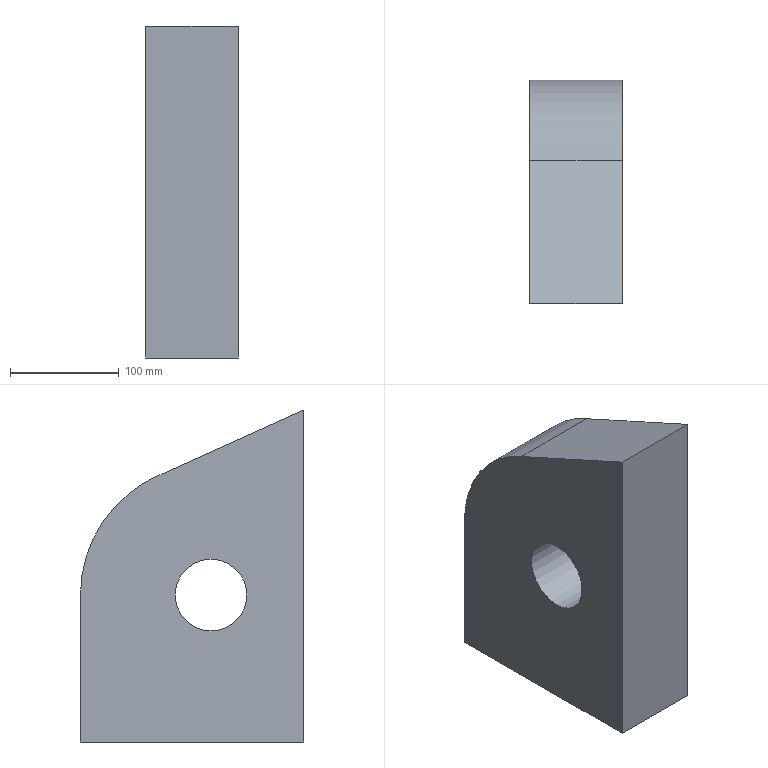Part | NX | features solid 2 | 1 solid | 8 faces | box 85 x 205 x 305 mm | volume 4128992 mm3 | plane 6 | cylinder 2 | commonest cylinder face diameters 66 x1 240 x1
STEP:
#1=CARTESIAN_POINT('',(1245.,1105.,-512.));
#2=VERTEX_POINT('',#1);
#3=CARTESIAN_POINT('',(1245.,1105.,-545.));
#4=DIRECTION('',(1.,0.,0.));
#5=DIRECTION('',(0.,0.,1.));
#6=AXIS2_PLACEMENT_3D('',#3,#4,#5);
#7=CIRCLE('',#6,33.);
#8=EDGE_CURVE('',#2,#2,#7,.F.);
#9=ORIENTED_EDGE('',*,*,#8,.T.);
#10=EDGE_LOOP('',(#9));
#11=FACE_BOUND('',#10,.T.);
#12=CARTESIAN_POINT('',(1330.,1105.,-512.));
#13=VERTEX_POINT('',#12);
#14=CARTESIAN_POINT('',(1330.,1105.,-545.));
#15=DIRECTION('',(1.,0.,0.));
#16=DIRECTION('',(0.,0.,1.));
#17=AXIS2_PLACEMENT_3D('',#14,#15,#16);
#18=CIRCLE('',#17,33.);
#19=EDGE_CURVE('',#13,#13,#18,.F.);
#20=ORIENTED_EDGE('',*,*,#19,.F.);
#21=EDGE_LOOP('',(#20));
#22=FACE_BOUND('',#21,.T.);
#23=CARTESIAN_POINT('',(1495.,1105.,-545.));
#24=DIRECTION('',(-1.,0.,0.));
#25=DIRECTION('',(0.,0.,-1.));
#26=AXIS2_PLACEMENT_3D('',#23,#24,#25);
#27=CYLINDRICAL_SURFACE('',#26,33.);
#28=ADVANCED_FACE('',(#11,#22),#27,.F.);
#29=CARTESIAN_POINT('',(1330.,1150.971,-434.155));
#30=VERTEX_POINT('',#29);
#31=CARTESIAN_POINT('',(1245.,1150.971,-434.155));
#32=VERTEX_POINT('',#31);
#33=CARTESIAN_POINT('',(1175.,1150.971,-434.155));
#34=DIRECTION('',(1.,0.,0.));
#35=VECTOR('',#34,1000.);
#36=LINE('',#33,#35);
#37=EDGE_CURVE('',#30,#32,#36,.F.);
#38=ORIENTED_EDGE('',*,*,#37,.F.);
#39=CARTESIAN_POINT('',(1330.,1225.,-545.));
#40=VERTEX_POINT('',#39);
#41=CARTESIAN_POINT('',(1330.,1105.,-545.));
#42=DIRECTION('',(1.,0.,0.));
#43=DIRECTION('',(0.,0.,1.));
#44=AXIS2_PLACEMENT_3D('',#41,#42,#43);
#45=CIRCLE('',#44,120.);
#46=EDGE_CURVE('',#40,#30,#45,.T.);
#47=ORIENTED_EDGE('',*,*,#46,.F.);
#48=CARTESIAN_POINT('',(1245.,1225.,-545.));
#49=VERTEX_POINT('',#48);
#50=CARTESIAN_POINT('',(1175.,1225.,-545.));
#51=DIRECTION('',(-1.,0.,0.));
#52=VECTOR('',#51,1000.);
#53=LINE('',#50,#52);
#54=EDGE_CURVE('',#49,#40,#53,.F.);
#55=ORIENTED_EDGE('',*,*,#54,.F.);
#56=CARTESIAN_POINT('',(1245.,1105.,-545.));
#57=DIRECTION('',(1.,0.,0.));
#58=DIRECTION('',(0.,0.,1.));
#59=AXIS2_PLACEMENT_3D('',#56,#57,#58);
#60=CIRCLE('',#59,120.);
#61=EDGE_CURVE('',#32,#49,#60,.F.);
#62=ORIENTED_EDGE('',*,*,#61,.F.);
#63=EDGE_LOOP('',(#38,#47,#55,#62));
#64=FACE_BOUND('',#63,.T.);
#65=CARTESIAN_POINT('',(1175.,1105.,-545.));
#66=DIRECTION('',(1.,0.,0.));
#67=DIRECTION('',(0.,0.,-1.));
#68=AXIS2_PLACEMENT_3D('',#65,#66,#67);
#69=CYLINDRICAL_SURFACE('',#68,120.);
#70=ADVANCED_FACE('',(#64),#69,.T.);
#71=CARTESIAN_POINT('',(1330.,1225.,-680.));
#72=VERTEX_POINT('',#71);
#73=CARTESIAN_POINT('',(1245.,1225.,-680.));
#74=VERTEX_POINT('',#73);
#75=CARTESIAN_POINT('',(1175.,1225.,-680.));
#76=DIRECTION('',(-1.,0.,0.));
#77=VECTOR('',#76,1000.);
#78=LINE('',#75,#77);
#79=EDGE_CURVE('',#72,#74,#78,.T.);
#80=ORIENTED_EDGE('',*,*,#79,.T.);
#81=CARTESIAN_POINT('',(1245.,1225.,-560.));
#82=DIRECTION('',(0.,0.,1.));
#83=VECTOR('',#82,1000.);
#84=LINE('',#81,#83);
#85=EDGE_CURVE('',#74,#49,#84,.T.);
#86=ORIENTED_EDGE('',*,*,#85,.T.);
#87=ORIENTED_EDGE('',*,*,#54,.T.);
#88=CARTESIAN_POINT('',(1330.,1225.,-560.));
#89=DIRECTION('',(0.,0.,1.));
#90=VECTOR('',#89,1000.);
#91=LINE('',#88,#90);
#92=EDGE_CURVE('',#72,#40,#91,.T.);
#93=ORIENTED_EDGE('',*,*,#92,.F.);
#94=EDGE_LOOP('',(#80,#86,#87,#93));
#95=FACE_BOUND('',#94,.T.);
#96=CARTESIAN_POINT('',(1175.,1225.,-560.));
#97=DIRECTION('',(0.,1.,0.));
#98=DIRECTION('',(-1.,0.,0.));
#99=AXIS2_PLACEMENT_3D('',#96,#97,#98);
#100=PLANE('',#99);
#101=ADVANCED_FACE('',(#95),#100,.T.);
#102=ORIENTED_EDGE('',*,*,#46,.T.);
#103=CARTESIAN_POINT('',(1330.,1020.,-375.));
#104=VERTEX_POINT('',#103);
#105=CARTESIAN_POINT('',(1330.,1177.538,-446.154));
#106=DIRECTION('',(0.,0.9114,-0.4116));
#107=VECTOR('',#106,1000.);
#108=LINE('',#105,#107);
#109=EDGE_CURVE('',#104,#30,#108,.T.);
#110=ORIENTED_EDGE('',*,*,#109,.F.);
#111=CARTESIAN_POINT('',(1330.,1020.,-680.));
#112=VERTEX_POINT('',#111);
#113=CARTESIAN_POINT('',(1330.,1020.,-360.));
#114=DIRECTION('',(0.,0.,-1.));
#115=VECTOR('',#114,1000.);
#116=LINE('',#113,#115);
#117=EDGE_CURVE('',#104,#112,#116,.T.);
#118=ORIENTED_EDGE('',*,*,#117,.T.);
#119=CARTESIAN_POINT('',(1330.,1050.,-680.));
#120=DIRECTION('',(0.,-1.,0.));
#121=VECTOR('',#120,1000.);
#122=LINE('',#119,#121);
#123=EDGE_CURVE('',#72,#112,#122,.T.);
#124=ORIENTED_EDGE('',*,*,#123,.F.);
#125=ORIENTED_EDGE('',*,*,#92,.T.);
#126=EDGE_LOOP('',(#102,#110,#118,#124,#125));
#127=FACE_BOUND('',#126,.T.);
#128=ORIENTED_EDGE('',*,*,#19,.T.);
#129=EDGE_LOOP('',(#128));
#130=FACE_BOUND('',#129,.T.);
#131=CARTESIAN_POINT('',(1330.,1050.,-510.));
#132=DIRECTION('',(-1.,0.,0.));
#133=DIRECTION('',(0.,-1.,0.));
#134=AXIS2_PLACEMENT_3D('',#131,#132,#133);
#135=PLANE('',#134);
#136=ADVANCED_FACE('',(#127,#130),#135,.F.);
#137=CARTESIAN_POINT('',(1245.,1020.,-375.));
#138=VERTEX_POINT('',#137);
#139=CARTESIAN_POINT('',(1245.,1038.757,-383.472));
#140=DIRECTION('',(0.,0.9114,-0.4116));
#141=VECTOR('',#140,1000.);
#142=LINE('',#139,#141);
#143=EDGE_CURVE('',#138,#32,#142,.T.);
#144=ORIENTED_EDGE('',*,*,#143,.T.);
#145=ORIENTED_EDGE('',*,*,#61,.T.);
#146=ORIENTED_EDGE('',*,*,#85,.F.);
#147=CARTESIAN_POINT('',(1245.,1020.,-680.));
#148=VERTEX_POINT('',#147);
#149=CARTESIAN_POINT('',(1245.,1020.,-680.));
#150=DIRECTION('',(0.,-1.,0.));
#151=VECTOR('',#150,1000.);
#152=LINE('',#149,#151);
#153=EDGE_CURVE('',#74,#148,#152,.T.);
#154=ORIENTED_EDGE('',*,*,#153,.T.);
#155=CARTESIAN_POINT('',(1245.,1020.,-501.379));
#156=DIRECTION('',(0.,0.,-1.));
#157=VECTOR('',#156,1000.);
#158=LINE('',#155,#157);
#159=EDGE_CURVE('',#148,#138,#158,.F.);
#160=ORIENTED_EDGE('',*,*,#159,.T.);
#161=EDGE_LOOP('',(#144,#145,#146,#154,#160));
#162=FACE_BOUND('',#161,.T.);
#163=ORIENTED_EDGE('',*,*,#8,.F.);
#164=EDGE_LOOP('',(#163));
#165=FACE_BOUND('',#164,.T.);
#166=CARTESIAN_POINT('',(1245.,1020.,-250.));
#167=DIRECTION('',(-1.,0.,0.));
#168=DIRECTION('',(0.,0.,-1.));
#169=AXIS2_PLACEMENT_3D('',#166,#167,#168);
#170=PLANE('',#169);
#171=ADVANCED_FACE('',(#162,#165),#170,.T.);
#172=CARTESIAN_POINT('',(1380.,1020.,-375.));
#173=DIRECTION('',(1.,0.,0.));
#174=VECTOR('',#173,1000.);
#175=LINE('',#172,#174);
#176=EDGE_CURVE('',#138,#104,#175,.T.);
#177=ORIENTED_EDGE('',*,*,#176,.F.);
#178=ORIENTED_EDGE('',*,*,#159,.F.);
#179=CARTESIAN_POINT('',(1550.,1020.,-680.));
#180=DIRECTION('',(1.,0.,0.));
#181=VECTOR('',#180,1000.);
#182=LINE('',#179,#181);
#183=EDGE_CURVE('',#148,#112,#182,.T.);
#184=ORIENTED_EDGE('',*,*,#183,.T.);
#185=ORIENTED_EDGE('',*,*,#117,.F.);
#186=EDGE_LOOP('',(#177,#178,#184,#185));
#187=FACE_BOUND('',#186,.T.);
#188=CARTESIAN_POINT('',(1550.,1020.,-425.));
#189=DIRECTION('',(0.,-1.,0.));
#190=DIRECTION('',(0.,0.,1.));
#191=AXIS2_PLACEMENT_3D('',#188,#189,#190);
#192=PLANE('',#191);
#193=ADVANCED_FACE('',(#187),#192,.T.);
#194=ORIENTED_EDGE('',*,*,#79,.F.);
#195=ORIENTED_EDGE('',*,*,#123,.T.);
#196=ORIENTED_EDGE('',*,*,#183,.F.);
#197=ORIENTED_EDGE('',*,*,#153,.F.);
#198=EDGE_LOOP('',(#194,#195,#196,#197));
#199=FACE_BOUND('',#198,.T.);
#200=CARTESIAN_POINT('',(80.,-155.,-680.));
#201=DIRECTION('',(0.,0.,1.));
#202=DIRECTION('',(-1.,0.,0.));
#203=AXIS2_PLACEMENT_3D('',#200,#201,#202);
#204=PLANE('',#203);
#205=ADVANCED_FACE('',(#199),#204,.F.);
#206=ORIENTED_EDGE('',*,*,#109,.T.);
#207=ORIENTED_EDGE('',*,*,#37,.T.);
#208=ORIENTED_EDGE('',*,*,#143,.F.);
#209=ORIENTED_EDGE('',*,*,#176,.T.);
#210=EDGE_LOOP('',(#206,#207,#208,#209));
#211=FACE_BOUND('',#210,.T.);
#212=CARTESIAN_POINT('',(1330.,1020.,-375.));
#213=DIRECTION('',(0.,0.4116,0.9114));
#214=DIRECTION('',(0.,0.9114,-0.4116));
#215=AXIS2_PLACEMENT_3D('',#212,#213,#214);
#216=PLANE('',#215);
#217=ADVANCED_FACE('',(#211),#216,.T.);
#218=CLOSED_SHELL('',(#28,#70,#101,#136,#171,#193,#205,#217));
#219=MANIFOLD_SOLID_BREP('',#218);
#220=(LENGTH_UNIT()NAMED_UNIT(*)SI_UNIT(.MILLI.,.METRE.));
#221=UNCERTAINTY_MEASURE_WITH_UNIT(LENGTH_MEASURE(0.00001),#220,'','');
#222=(NAMED_UNIT(*)PLANE_ANGLE_UNIT()SI_UNIT($,.RADIAN.));
#223=(NAMED_UNIT(*)SI_UNIT($,.STERADIAN.)SOLID_ANGLE_UNIT());
#224=(GEOMETRIC_REPRESENTATION_CONTEXT(3)GLOBAL_UNCERTAINTY_ASSIGNED_CONTEXT((#221))GLOBAL_UNIT_ASSIGNED_CONTEXT((#220,#222,#223))REPRESENTATION_CONTEXT('',''));
#225=ADVANCED_BREP_SHAPE_REPRESENTATION('',(#219),#224);